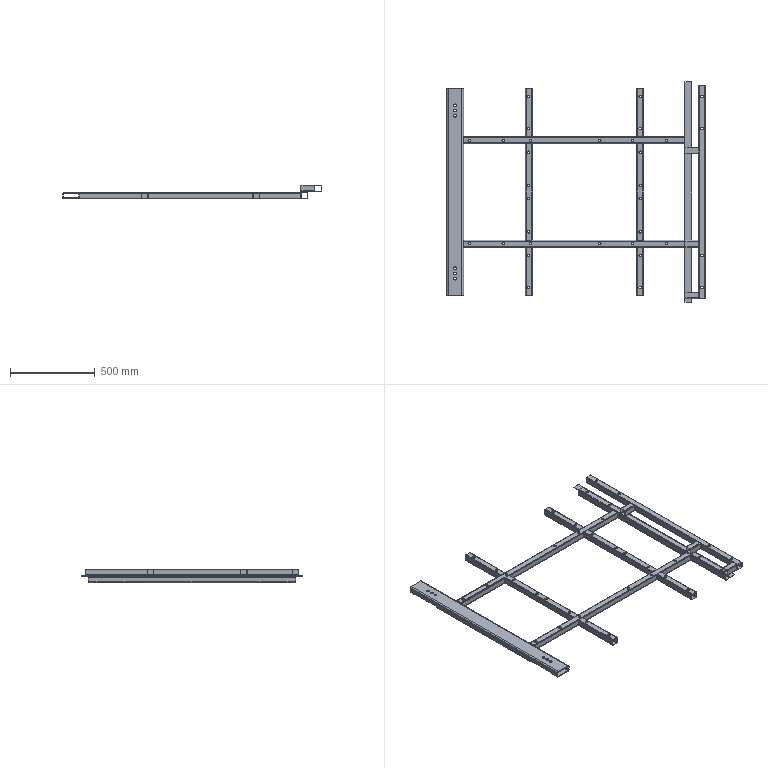Part | NX | features BREP 8 | 16 solids | 678 faces | box 1524 x 1300 x 82 mm | volume 3863519 mm3 | cylinder 366 | plane 312 | commonest cylinder face diameters 15 x144 6 x112 10 x56 8 x20 20 x14 17 x12